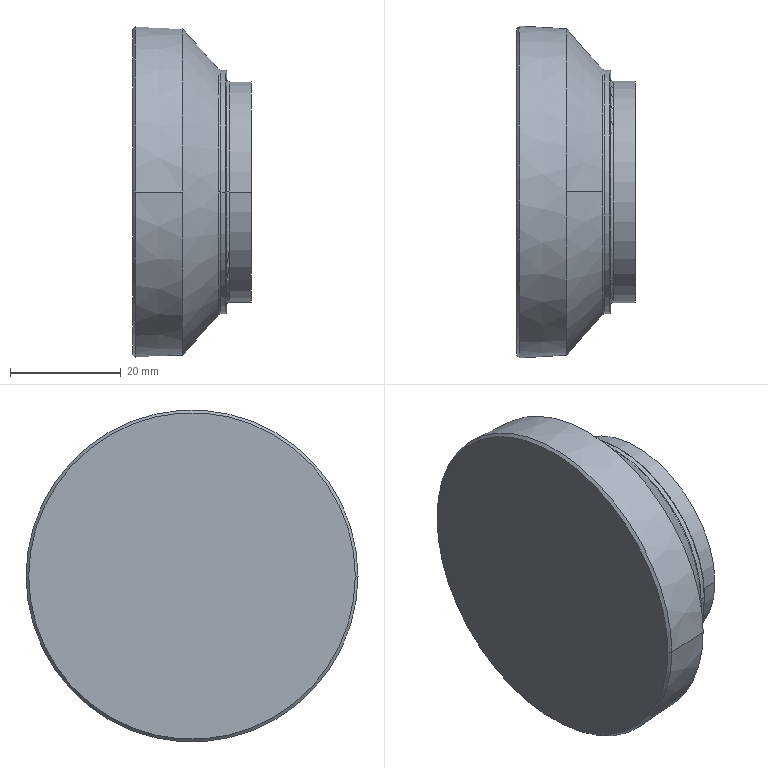Part | SolidWorks | features BaseBody 1 | 1 solid | 23 faces | box 21.5 x 60 x 60 mm | volume 41869 mm3 | torus 6 | cone 6 | cylinder 6 | plane 3 | sphere 2 | commonest cylinder face diameters 22 x2 40 x2 44 x2
STEP:
#1=CARTESIAN_POINT('',(-11.027,-22.,0.));
#2=VERTEX_POINT('',#1);
#3=CARTESIAN_POINT('',(-11.027,22.,0.));
#4=VERTEX_POINT('',#3);
#5=CARTESIAN_POINT('',(-11.027,0.,0.));
#6=DIRECTION('',(1.,0.,0.));
#7=DIRECTION('',(0.,0.,-1.));
#8=AXIS2_PLACEMENT_3D('',#5,#6,#7);
#9=CIRCLE('',#8,22.);
#10=EDGE_CURVE('',#2,#4,#9,.T.);
#11=ORIENTED_EDGE('',*,*,#10,.F.);
#12=CARTESIAN_POINT('',(-11.399,-22.166,0.));
#13=VERTEX_POINT('',#12);
#14=CARTESIAN_POINT('',(-11.027,-22.5,0.));
#15=DIRECTION('',(0.,0.,1.));
#16=DIRECTION('',(0.,-1.,0.));
#17=AXIS2_PLACEMENT_3D('',#14,#15,#16);
#18=CIRCLE('',#17,0.5);
#19=EDGE_CURVE('',#2,#13,#18,.T.);
#20=ORIENTED_EDGE('',*,*,#19,.T.);
#21=CARTESIAN_POINT('',(-11.399,0.,-22.166));
#22=VERTEX_POINT('',#21);
#23=CARTESIAN_POINT('',(-11.399,0.,0.));
#24=DIRECTION('',(-1.,0.,0.));
#25=DIRECTION('',(0.,-1.,0.));
#26=AXIS2_PLACEMENT_3D('',#23,#24,#25);
#27=CIRCLE('',#26,22.166);
#28=EDGE_CURVE('',#22,#13,#27,.T.);
#29=ORIENTED_EDGE('',*,*,#28,.F.);
#30=CARTESIAN_POINT('',(-11.399,22.166,0.));
#31=VERTEX_POINT('',#30);
#32=CARTESIAN_POINT('',(-11.399,0.,0.));
#33=DIRECTION('',(-1.,0.,0.));
#34=DIRECTION('',(0.,-1.,0.));
#35=AXIS2_PLACEMENT_3D('',#32,#33,#34);
#36=CIRCLE('',#35,22.166);
#37=EDGE_CURVE('',#31,#22,#36,.T.);
#38=ORIENTED_EDGE('',*,*,#37,.F.);
#39=CARTESIAN_POINT('',(-11.027,22.5,0.));
#40=DIRECTION('',(0.,0.,-1.));
#41=DIRECTION('',(-1.,0.,0.));
#42=AXIS2_PLACEMENT_3D('',#39,#40,#41);
#43=CIRCLE('',#42,0.5);
#44=EDGE_CURVE('',#4,#31,#43,.T.);
#45=ORIENTED_EDGE('',*,*,#44,.F.);
#46=EDGE_LOOP('',(#11,#20,#29,#38,#45));
#47=FACE_OUTER_BOUND('',#46,.T.);
#48=CARTESIAN_POINT('',(-11.027,0.,0.));
#49=DIRECTION('',(1.,0.,0.));
#50=DIRECTION('',(0.,1.,0.));
#51=AXIS2_PLACEMENT_3D('',#48,#49,#50);
#52=TOROIDAL_SURFACE('',#51,22.5,0.5);
#53=ADVANCED_FACE('',(#47),#52,.F.);
#54=CARTESIAN_POINT('',(-10.2,-22.,0.));
#55=VERTEX_POINT('',#54);
#56=CARTESIAN_POINT('',(-10.2,22.,0.));
#57=VERTEX_POINT('',#56);
#58=CARTESIAN_POINT('',(-10.2,0.,0.));
#59=DIRECTION('',(-1.,0.,0.));
#60=DIRECTION('',(0.,-1.,0.));
#61=AXIS2_PLACEMENT_3D('',#58,#59,#60);
#62=CIRCLE('',#61,22.);
#63=EDGE_CURVE('',#55,#57,#62,.T.);
#64=ORIENTED_EDGE('',*,*,#63,.F.);
#65=CARTESIAN_POINT('',(-10.,-21.8,0.));
#66=VERTEX_POINT('',#65);
#67=CARTESIAN_POINT('',(-10.2,-21.8,0.));
#68=DIRECTION('',(0.,0.,1.));
#69=DIRECTION('',(0.,-1.,0.));
#70=AXIS2_PLACEMENT_3D('',#67,#68,#69);
#71=CIRCLE('',#70,0.2);
#72=EDGE_CURVE('',#55,#66,#71,.T.);
#73=ORIENTED_EDGE('',*,*,#72,.T.);
#74=CARTESIAN_POINT('',(-10.,21.8,0.));
#75=VERTEX_POINT('',#74);
#76=CARTESIAN_POINT('',(-10.,0.,0.));
#77=DIRECTION('',(-1.,0.,0.));
#78=DIRECTION('',(0.,-1.,0.));
#79=AXIS2_PLACEMENT_3D('',#76,#77,#78);
#80=CIRCLE('',#79,21.8);
#81=EDGE_CURVE('',#66,#75,#80,.T.);
#82=ORIENTED_EDGE('',*,*,#81,.T.);
#83=CARTESIAN_POINT('',(-10.2,21.8,0.));
#84=DIRECTION('',(0.,0.,-1.));
#85=DIRECTION('',(-1.,0.,0.));
#86=AXIS2_PLACEMENT_3D('',#83,#84,#85);
#87=CIRCLE('',#86,0.2);
#88=EDGE_CURVE('',#57,#75,#87,.T.);
#89=ORIENTED_EDGE('',*,*,#88,.F.);
#90=EDGE_LOOP('',(#64,#73,#82,#89));
#91=FACE_OUTER_BOUND('',#90,.T.);
#92=CARTESIAN_POINT('',(-10.2,0.,0.));
#93=DIRECTION('',(1.,0.,0.));
#94=DIRECTION('',(0.,1.,0.));
#95=AXIS2_PLACEMENT_3D('',#92,#93,#94);
#96=TOROIDAL_SURFACE('',#95,21.8,0.2);
#97=ADVANCED_FACE('',(#91),#96,.T.);
#98=CARTESIAN_POINT('',(-9.5,-20.,0.));
#99=VERTEX_POINT('',#98);
#100=CARTESIAN_POINT('',(-9.5,20.,0.));
#101=VERTEX_POINT('',#100);
#102=CARTESIAN_POINT('',(-9.5,0.,0.));
#103=DIRECTION('',(1.,0.,0.));
#104=DIRECTION('',(0.,0.,-1.));
#105=AXIS2_PLACEMENT_3D('',#102,#103,#104);
#106=CIRCLE('',#105,20.);
#107=EDGE_CURVE('',#99,#101,#106,.T.);
#108=ORIENTED_EDGE('',*,*,#107,.F.);
#109=CARTESIAN_POINT('',(-10.,-20.5,0.));
#110=VERTEX_POINT('',#109);
#111=CARTESIAN_POINT('',(-9.5,-20.5,0.));
#112=DIRECTION('',(0.,0.,1.));
#113=DIRECTION('',(0.,-1.,0.));
#114=AXIS2_PLACEMENT_3D('',#111,#112,#113);
#115=CIRCLE('',#114,0.5);
#116=EDGE_CURVE('',#99,#110,#115,.T.);
#117=ORIENTED_EDGE('',*,*,#116,.T.);
#118=CARTESIAN_POINT('',(-10.,0.,-20.5));
#119=VERTEX_POINT('',#118);
#120=CARTESIAN_POINT('',(-10.,0.,-20.5));
#121=CARTESIAN_POINT('',(-10.,-0.627,-20.5));
#122=CARTESIAN_POINT('',(-10.,-1.564,-20.457));
#123=CARTESIAN_POINT('',(-10.,-2.649,-20.332));
#124=CARTESIAN_POINT('',(-10.,-3.19,-20.251));
#125=CARTESIAN_POINT('',(-10.,-3.46,-20.206));
#126=CARTESIAN_POINT('',(-10.,-3.595,-20.182));
#127=CARTESIAN_POINT('',(-10.,-3.653,-20.172));
#128=CARTESIAN_POINT('',(-10.,-3.692,-20.165));
#129=CARTESIAN_POINT('',(-10.,-3.71,-20.162));
#130=CARTESIAN_POINT('',(-10.,-4.384,-20.037));
#131=CARTESIAN_POINT('',(-10.,-5.351,-19.809));
#132=CARTESIAN_POINT('',(-10.,-6.456,-19.462));
#133=CARTESIAN_POINT('',(-10.,-7.003,-19.268));
#134=CARTESIAN_POINT('',(-10.,-7.275,-19.166));
#135=CARTESIAN_POINT('',(-10.,-7.391,-19.121));
#136=CARTESIAN_POINT('',(-10.,-7.469,-19.091));
#137=CARTESIAN_POINT('',(-10.,-7.506,-19.077));
#138=CARTESIAN_POINT('',(-10.,-8.19,-18.806));
#139=CARTESIAN_POINT('',(-10.,-9.132,-18.377));
#140=CARTESIAN_POINT('',(-10.,-10.189,-17.795));
#141=CARTESIAN_POINT('',(-10.,-10.707,-17.483));
#142=CARTESIAN_POINT('',(-10.,-10.927,-17.346));
#143=CARTESIAN_POINT('',(-10.,-11.073,-17.253));
#144=CARTESIAN_POINT('',(-10.,-11.144,-17.207));
#145=CARTESIAN_POINT('',(-10.,-12.402,-16.384));
#146=CARTESIAN_POINT('',(-10.,-13.495,-15.496));
#147=CARTESIAN_POINT('',(-10.,-14.996,-13.995));
#148=CARTESIAN_POINT('',(-10.,-15.704,-13.211));
#149=CARTESIAN_POINT('',(-10.,-16.456,-12.234));
#150=CARTESIAN_POINT('',(-10.,-16.813,-11.731));
#151=CARTESIAN_POINT('',(-10.,-16.963,-11.512));
#152=CARTESIAN_POINT('',(-10.,-17.061,-11.366));
#153=CARTESIAN_POINT('',(-10.,-17.111,-11.29));
#154=CARTESIAN_POINT('',(-10.,-17.537,-10.638));
#155=CARTESIAN_POINT('',(-10.,-18.059,-9.744));
#156=CARTESIAN_POINT('',(-10.,-18.587,-8.659));
#157=CARTESIAN_POINT('',(-10.,-18.831,-8.106));
#158=CARTESIAN_POINT('',(-10.,-18.947,-7.827));
#159=CARTESIAN_POINT('',(-10.,-18.996,-7.707));
#160=CARTESIAN_POINT('',(-10.,-19.029,-7.626));
#161=CARTESIAN_POINT('',(-10.,-19.045,-7.585));
#162=CARTESIAN_POINT('',(-10.,-19.305,-6.928));
#163=CARTESIAN_POINT('',(-10.,-19.626,-5.987));
#164=CARTESIAN_POINT('',(-10.,-19.919,-4.867));
#165=CARTESIAN_POINT('',(-10.,-20.045,-4.3));
#166=CARTESIAN_POINT('',(-10.,-20.103,-4.016));
#167=CARTESIAN_POINT('',(-10.,-20.131,-3.873));
#168=CARTESIAN_POINT('',(-10.,-20.142,-3.812));
#169=CARTESIAN_POINT('',(-10.,-20.15,-3.771));
#170=CARTESIAN_POINT('',(-10.,-20.154,-3.749));
#171=CARTESIAN_POINT('',(-10.,-20.386,-2.498));
#172=CARTESIAN_POINT('',(-10.,-20.5,-1.254));
#173=CARTESIAN_POINT('',(-10.,-20.5,0.));
#174=B_SPLINE_CURVE_WITH_KNOTS('',3,(#120,#121,#122,#123,#124,#125,#126,#127,#128,#129,#130,#131,#132,#133,#134,#135,#136,#137,#138,#139,#140,#141,#142,#143,#144,#145,#146,#147,#148,#149,#150,#151,#152,#153,#154,#155,#156,#157,#158,#159,#160,#161,#162,#163,#164,#165,#166,#167,#168,#169,#170,#171,#172,#173),.UNSPECIFIED.,.F.,.F.,(4,1,1,1,1,1,2,2,1,1,1,1,2,2,1,1,1,2,2,2,1,1,1,2,2,1,1,1,1,2,2,1,1,1,1,1,2,2,4),(0.,0.0625,0.09375,0.1094,0.1172,0.1211,0.123,0.125,0.1875,0.2187,0.2344,0.2422,0.2461,0.25,0.3125,0.3437,0.3594,0.3672,0.375,0.5,0.5625,0.5938,0.6094,0.6172,0.625,0.6875,0.7188,0.7344,0.7422,0.7461,0.75,0.8125,0.8438,0.8594,0.8672,0.8711,0.873,0.875,1.),.UNSPECIFIED.);
#175=EDGE_CURVE('',#119,#110,#174,.T.);
#176=ORIENTED_EDGE('',*,*,#175,.F.);
#177=CARTESIAN_POINT('',(-10.,20.5,0.));
#178=VERTEX_POINT('',#177);
#179=CARTESIAN_POINT('',(-10.,20.5,0.));
#180=CARTESIAN_POINT('',(-10.,20.5,-0.6268));
#181=CARTESIAN_POINT('',(-10.,20.457,-1.563));
#182=CARTESIAN_POINT('',(-10.,20.332,-2.649));
#183=CARTESIAN_POINT('',(-10.,20.251,-3.19));
#184=CARTESIAN_POINT('',(-10.,20.206,-3.46));
#185=CARTESIAN_POINT('',(-10.,20.182,-3.595));
#186=CARTESIAN_POINT('',(-10.,20.172,-3.653));
#187=CARTESIAN_POINT('',(-10.,20.165,-3.692));
#188=CARTESIAN_POINT('',(-10.,20.162,-3.71));
#189=CARTESIAN_POINT('',(-10.,20.037,-4.384));
#190=CARTESIAN_POINT('',(-10.,19.809,-5.351));
#191=CARTESIAN_POINT('',(-10.,19.462,-6.456));
#192=CARTESIAN_POINT('',(-10.,19.268,-7.003));
#193=CARTESIAN_POINT('',(-10.,19.166,-7.275));
#194=CARTESIAN_POINT('',(-10.,19.121,-7.391));
#195=CARTESIAN_POINT('',(-10.,19.091,-7.469));
#196=CARTESIAN_POINT('',(-10.,19.077,-7.506));
#197=CARTESIAN_POINT('',(-10.,18.806,-8.19));
#198=CARTESIAN_POINT('',(-10.,18.377,-9.132));
#199=CARTESIAN_POINT('',(-10.,17.795,-10.189));
#200=CARTESIAN_POINT('',(-10.,17.483,-10.707));
#201=CARTESIAN_POINT('',(-10.,17.346,-10.927));
#202=CARTESIAN_POINT('',(-10.,17.253,-11.073));
#203=CARTESIAN_POINT('',(-10.,17.207,-11.144));
#204=CARTESIAN_POINT('',(-10.,16.384,-12.402));
#205=CARTESIAN_POINT('',(-10.,15.496,-13.495));
#206=CARTESIAN_POINT('',(-10.,13.995,-14.996));
#207=CARTESIAN_POINT('',(-10.,13.211,-15.704));
#208=CARTESIAN_POINT('',(-10.,12.234,-16.456));
#209=CARTESIAN_POINT('',(-10.,11.731,-16.813));
#210=CARTESIAN_POINT('',(-10.,11.512,-16.963));
#211=CARTESIAN_POINT('',(-10.,11.366,-17.061));
#212=CARTESIAN_POINT('',(-10.,11.29,-17.111));
#213=CARTESIAN_POINT('',(-10.,10.638,-17.537));
#214=CARTESIAN_POINT('',(-10.,9.744,-18.059));
#215=CARTESIAN_POINT('',(-10.,8.659,-18.587));
#216=CARTESIAN_POINT('',(-10.,8.106,-18.831));
#217=CARTESIAN_POINT('',(-10.,7.827,-18.947));
#218=CARTESIAN_POINT('',(-10.,7.707,-18.996));
#219=CARTESIAN_POINT('',(-10.,7.626,-19.029));
#220=CARTESIAN_POINT('',(-10.,7.585,-19.045));
#221=CARTESIAN_POINT('',(-10.,6.928,-19.305));
#222=CARTESIAN_POINT('',(-10.,5.987,-19.626));
#223=CARTESIAN_POINT('',(-10.,4.867,-19.919));
#224=CARTESIAN_POINT('',(-10.,4.3,-20.045));
#225=CARTESIAN_POINT('',(-10.,4.016,-20.103));
#226=CARTESIAN_POINT('',(-10.,3.873,-20.131));
#227=CARTESIAN_POINT('',(-10.,3.812,-20.142));
#228=CARTESIAN_POINT('',(-10.,3.771,-20.15));
#229=CARTESIAN_POINT('',(-10.,3.749,-20.154));
#230=CARTESIAN_POINT('',(-10.,2.498,-20.386));
#231=CARTESIAN_POINT('',(-10.,1.254,-20.5));
#232=CARTESIAN_POINT('',(-10.,0.,-20.5));
#233=B_SPLINE_CURVE_WITH_KNOTS('',3,(#179,#180,#181,#182,#183,#184,#185,#186,#187,#188,#189,#190,#191,#192,#193,#194,#195,#196,#197,#198,#199,#200,#201,#202,#203,#204,#205,#206,#207,#208,#209,#210,#211,#212,#213,#214,#215,#216,#217,#218,#219,#220,#221,#222,#223,#224,#225,#226,#227,#228,#229,#230,#231,#232),.UNSPECIFIED.,.F.,.F.,(4,1,1,1,1,1,2,2,1,1,1,1,2,2,1,1,1,2,2,2,1,1,1,2,2,1,1,1,1,2,2,1,1,1,1,1,2,2,4),(0.5,0.5312,0.5469,0.5547,0.5586,0.5605,0.5615,0.5625,0.5937,0.6094,0.6172,0.6211,0.623,0.625,0.6562,0.6719,0.6797,0.6836,0.6875,0.75,0.7812,0.7969,0.8047,0.8086,0.8125,0.8437,0.8594,0.8672,0.8711,0.873,0.875,0.9062,0.9219,0.9297,0.9336,0.9355,0.9365,0.9375,1.),.UNSPECIFIED.);
#234=EDGE_CURVE('',#178,#119,#233,.T.);
#235=ORIENTED_EDGE('',*,*,#234,.F.);
#236=CARTESIAN_POINT('',(-9.5,20.5,0.));
#237=DIRECTION('',(0.,0.,-1.));
#238=DIRECTION('',(-1.,0.,0.));
#239=AXIS2_PLACEMENT_3D('',#236,#237,#238);
#240=CIRCLE('',#239,0.5);
#241=EDGE_CURVE('',#101,#178,#240,.T.);
#242=ORIENTED_EDGE('',*,*,#241,.F.);
#243=EDGE_LOOP('',(#108,#117,#176,#235,#242));
#244=FACE_OUTER_BOUND('',#243,.T.);
#245=CARTESIAN_POINT('',(-9.5,0.,0.));
#246=DIRECTION('',(1.,0.,0.));
#247=DIRECTION('',(0.,1.,0.));
#248=AXIS2_PLACEMENT_3D('',#245,#246,#247);
#249=TOROIDAL_SURFACE('',#248,20.5,0.5);
#250=ADVANCED_FACE('',(#244),#249,.F.);
#251=CARTESIAN_POINT('',(-22.,0.,0.));
#252=VERTEX_POINT('',#251);
#253=CARTESIAN_POINT('',(-11.,11.,0.));
#254=VERTEX_POINT('',#253);
#255=CARTESIAN_POINT('',(-11.,0.,0.));
#256=DIRECTION('',(0.,0.,-1.));
#257=DIRECTION('',(-1.,0.,0.));
#258=AXIS2_PLACEMENT_3D('',#255,#256,#257);
#259=CIRCLE('',#258,11.);
#260=EDGE_CURVE('',#252,#254,#259,.T.);
#261=ORIENTED_EDGE('',*,*,#260,.F.);
#262=CARTESIAN_POINT('',(-11.,-11.,0.));
#263=VERTEX_POINT('',#262);
#264=CARTESIAN_POINT('',(-11.,0.,0.));
#265=DIRECTION('',(0.,0.,1.));
#266=DIRECTION('',(1.,0.,0.));
#267=AXIS2_PLACEMENT_3D('',#264,#265,#266);
#268=CIRCLE('',#267,11.);
#269=EDGE_CURVE('',#252,#263,#268,.T.);
#270=ORIENTED_EDGE('',*,*,#269,.T.);
#271=CARTESIAN_POINT('',(-11.,0.,0.));
#272=DIRECTION('',(1.,0.,0.));
#273=DIRECTION('',(0.,-1.,0.));
#274=AXIS2_PLACEMENT_3D('',#271,#272,#273);
#275=CIRCLE('',#274,11.);
#276=EDGE_CURVE('',#263,#254,#275,.T.);
#277=ORIENTED_EDGE('',*,*,#276,.T.);
#278=EDGE_LOOP('',(#261,#270,#277));
#279=FACE_OUTER_BOUND('',#278,.T.);
#280=CARTESIAN_POINT('',(-11.,0.,0.));
#281=DIRECTION('',(0.,0.,1.));
#282=DIRECTION('',(0.,1.,0.));
#283=AXIS2_PLACEMENT_3D('',#280,#281,#282);
#284=SPHERICAL_SURFACE('',#283,11.);
#285=ADVANCED_FACE('',(#279),#284,.F.);
#286=CARTESIAN_POINT('',(-27.,-29.5,0.));
#287=VERTEX_POINT('',#286);
#288=CARTESIAN_POINT('',(-27.,29.5,0.));
#289=VERTEX_POINT('',#288);
#290=CARTESIAN_POINT('',(-27.,0.,0.));
#291=DIRECTION('',(-1.,0.,0.));
#292=DIRECTION('',(0.,0.,-1.));
#293=AXIS2_PLACEMENT_3D('',#290,#291,#292);
#294=CIRCLE('',#293,29.5);
#295=EDGE_CURVE('',#287,#289,#294,.T.);
#296=ORIENTED_EDGE('',*,*,#295,.F.);
#297=CARTESIAN_POINT('',(-26.5,-30.,0.));
#298=VERTEX_POINT('',#297);
#299=CARTESIAN_POINT('',(-26.5,-30.,0.));
#300=DIRECTION('',(0.7071,-0.7071,0.));
#301=VECTOR('',#300,1000.);
#302=LINE('',#299,#301);
#303=EDGE_CURVE('',#287,#298,#302,.T.);
#304=ORIENTED_EDGE('',*,*,#303,.T.);
#305=CARTESIAN_POINT('',(-26.5,30.,0.));
#306=VERTEX_POINT('',#305);
#307=CARTESIAN_POINT('',(-26.5,0.,0.));
#308=DIRECTION('',(-1.,0.,0.));
#309=DIRECTION('',(0.,-1.,0.));
#310=AXIS2_PLACEMENT_3D('',#307,#308,#309);
#311=CIRCLE('',#310,30.);
#312=EDGE_CURVE('',#298,#306,#311,.T.);
#313=ORIENTED_EDGE('',*,*,#312,.T.);
#314=CARTESIAN_POINT('',(-26.5,30.,0.));
#315=DIRECTION('',(0.7071,0.7071,0.));
#316=VECTOR('',#315,1000.);
#317=LINE('',#314,#316);
#318=EDGE_CURVE('',#289,#306,#317,.T.);
#319=ORIENTED_EDGE('',*,*,#318,.F.);
#320=EDGE_LOOP('',(#296,#304,#313,#319));
#321=FACE_OUTER_BOUND('',#320,.T.);
#322=CARTESIAN_POINT('',(-26.5,0.,0.));
#323=DIRECTION('',(1.,0.,0.));
#324=DIRECTION('',(0.,1.,0.));
#325=AXIS2_PLACEMENT_3D('',#322,#323,#324);
#326=CONICAL_SURFACE('',#325,30.,0.7854);
#327=ADVANCED_FACE('',(#321),#326,.T.);
#328=CARTESIAN_POINT('',(-18.,0.,29.5));
#329=VERTEX_POINT('',#328);
#330=CARTESIAN_POINT('',(-18.,29.5,0.));
#331=VERTEX_POINT('',#330);
#332=CARTESIAN_POINT('',(-18.,0.,0.));
#333=DIRECTION('',(-1.,0.,0.));
#334=DIRECTION('',(0.,-1.,0.));
#335=AXIS2_PLACEMENT_3D('',#332,#333,#334);
#336=CIRCLE('',#335,29.5);
#337=EDGE_CURVE('',#329,#331,#336,.T.);
#338=ORIENTED_EDGE('',*,*,#337,.T.);
#339=CARTESIAN_POINT('',(-26.5,30.,0.));
#340=DIRECTION('',(-0.9983,0.05872,0.));
#341=VECTOR('',#340,1000.);
#342=LINE('',#339,#341);
#343=EDGE_CURVE('',#331,#306,#342,.T.);
#344=ORIENTED_EDGE('',*,*,#343,.T.);
#345=ORIENTED_EDGE('',*,*,#312,.F.);
#346=CARTESIAN_POINT('',(-18.,-29.5,0.));
#347=VERTEX_POINT('',#346);
#348=CARTESIAN_POINT('',(-26.5,-30.,0.));
#349=DIRECTION('',(-0.9983,-0.05872,0.));
#350=VECTOR('',#349,1000.);
#351=LINE('',#348,#350);
#352=EDGE_CURVE('',#347,#298,#351,.T.);
#353=ORIENTED_EDGE('',*,*,#352,.F.);
#354=CARTESIAN_POINT('',(-18.,0.,0.));
#355=DIRECTION('',(-1.,0.,0.));
#356=DIRECTION('',(0.,-1.,0.));
#357=AXIS2_PLACEMENT_3D('',#354,#355,#356);
#358=CIRCLE('',#357,29.5);
#359=EDGE_CURVE('',#347,#329,#358,.T.);
#360=ORIENTED_EDGE('',*,*,#359,.T.);
#361=EDGE_LOOP('',(#338,#344,#345,#353,#360));
#362=FACE_OUTER_BOUND('',#361,.T.);
#363=CARTESIAN_POINT('',(-26.5,0.,0.));
#364=DIRECTION('',(-1.,0.,0.));
#365=DIRECTION('',(0.,-1.,0.));
#366=AXIS2_PLACEMENT_3D('',#363,#364,#365);
#367=CONICAL_SURFACE('',#366,30.,0.05876);
#368=ADVANCED_FACE('',(#362),#367,.T.);
#369=CARTESIAN_POINT('',(-11.399,0.,22.166));
#370=VERTEX_POINT('',#369);
#371=CARTESIAN_POINT('',(-11.399,0.,0.));
#372=DIRECTION('',(-1.,0.,0.));
#373=DIRECTION('',(0.,-1.,0.));
#374=AXIS2_PLACEMENT_3D('',#371,#372,#373);
#375=CIRCLE('',#374,22.166);
#376=EDGE_CURVE('',#370,#31,#375,.T.);
#377=ORIENTED_EDGE('',*,*,#376,.T.);
#378=ORIENTED_EDGE('',*,*,#37,.T.);
#379=CARTESIAN_POINT('',(-18.,0.,-29.5));
#380=VERTEX_POINT('',#379);
#381=CARTESIAN_POINT('',(-18.,0.,-29.5));
#382=DIRECTION('',(-0.669,0.,-0.7433));
#383=VECTOR('',#382,1000.);
#384=LINE('',#381,#383);
#385=EDGE_CURVE('',#22,#380,#384,.T.);
#386=ORIENTED_EDGE('',*,*,#385,.T.);
#387=CARTESIAN_POINT('',(-18.,0.,0.));
#388=DIRECTION('',(-1.,0.,0.));
#389=DIRECTION('',(0.,-1.,0.));
#390=AXIS2_PLACEMENT_3D('',#387,#388,#389);
#391=CIRCLE('',#390,29.5);
#392=EDGE_CURVE('',#331,#380,#391,.T.);
#393=ORIENTED_EDGE('',*,*,#392,.F.);
#394=ORIENTED_EDGE('',*,*,#337,.F.);
#395=CARTESIAN_POINT('',(-18.,0.,29.5));
#396=DIRECTION('',(-0.669,0.,0.7433));
#397=VECTOR('',#396,1000.);
#398=LINE('',#395,#397);
#399=EDGE_CURVE('',#370,#329,#398,.T.);
#400=ORIENTED_EDGE('',*,*,#399,.F.);
#401=EDGE_LOOP('',(#377,#378,#386,#393,#394,#400));
#402=FACE_OUTER_BOUND('',#401,.T.);
#403=CARTESIAN_POINT('',(-18.,0.,0.));
#404=DIRECTION('',(-1.,0.,0.));
#405=DIRECTION('',(0.,0.,1.));
#406=AXIS2_PLACEMENT_3D('',#403,#404,#405);
#407=CONICAL_SURFACE('',#406,29.5,0.838);
#408=ADVANCED_FACE('',(#402),#407,.T.);
#409=ORIENTED_EDGE('',*,*,#63,.T.);
#410=CARTESIAN_POINT('',(-10.614,22.,0.));
#411=DIRECTION('',(-1.,0.,0.));
#412=VECTOR('',#411,1000.);
#413=LINE('',#410,#412);
#414=EDGE_CURVE('',#57,#4,#413,.T.);
#415=ORIENTED_EDGE('',*,*,#414,.T.);
#416=CARTESIAN_POINT('',(-11.027,0.,0.));
#417=DIRECTION('',(1.,0.,0.));
#418=DIRECTION('',(0.,0.,-1.));
#419=AXIS2_PLACEMENT_3D('',#416,#417,#418);
#420=CIRCLE('',#419,22.);
#421=EDGE_CURVE('',#4,#2,#420,.T.);
#422=ORIENTED_EDGE('',*,*,#421,.T.);
#423=CARTESIAN_POINT('',(-10.614,-22.,0.));
#424=DIRECTION('',(-1.,0.,0.));
#425=VECTOR('',#424,1000.);
#426=LINE('',#423,#425);
#427=EDGE_CURVE('',#55,#2,#426,.T.);
#428=ORIENTED_EDGE('',*,*,#427,.F.);
#429=EDGE_LOOP('',(#409,#415,#422,#428));
#430=FACE_OUTER_BOUND('',#429,.T.);
#431=CARTESIAN_POINT('',(-10.614,0.,0.));
#432=DIRECTION('',(-1.,0.,0.));
#433=DIRECTION('',(0.,-1.,0.));
#434=AXIS2_PLACEMENT_3D('',#431,#432,#433);
#435=CYLINDRICAL_SURFACE('',#434,22.);
#436=ADVANCED_FACE('',(#430),#435,.T.);
#437=CARTESIAN_POINT('',(-5.5,-20.,0.));
#438=VERTEX_POINT('',#437);
#439=CARTESIAN_POINT('',(-5.5,20.,0.));
#440=VERTEX_POINT('',#439);
#441=CARTESIAN_POINT('',(-5.5,0.,0.));
#442=DIRECTION('',(-1.,0.,0.));
#443=DIRECTION('',(0.,-1.,0.));
#444=AXIS2_PLACEMENT_3D('',#441,#442,#443);
#445=CIRCLE('',#444,20.);
#446=EDGE_CURVE('',#438,#440,#445,.T.);
#447=ORIENTED_EDGE('',*,*,#446,.T.);
#448=CARTESIAN_POINT('',(-7.5,20.,0.));
#449=DIRECTION('',(-1.,0.,0.));
#450=VECTOR('',#449,1000.);
#451=LINE('',#448,#450);
#452=EDGE_CURVE('',#440,#101,#451,.T.);
#453=ORIENTED_EDGE('',*,*,#452,.T.);
#454=CARTESIAN_POINT('',(-9.5,0.,0.));
#455=DIRECTION('',(1.,0.,0.));
#456=DIRECTION('',(0.,0.,-1.));
#457=AXIS2_PLACEMENT_3D('',#454,#455,#456);
#458=CIRCLE('',#457,20.);
#459=EDGE_CURVE('',#101,#99,#458,.T.);
#460=ORIENTED_EDGE('',*,*,#459,.T.);
#461=CARTESIAN_POINT('',(-7.5,-20.,0.));
#462=DIRECTION('',(-1.,0.,0.));
#463=VECTOR('',#462,1000.);
#464=LINE('',#461,#463);
#465=EDGE_CURVE('',#438,#99,#464,.T.);
#466=ORIENTED_EDGE('',*,*,#465,.F.);
#467=EDGE_LOOP('',(#447,#453,#460,#466));
#468=FACE_OUTER_BOUND('',#467,.T.);
#469=CARTESIAN_POINT('',(-7.5,0.,0.));
#470=DIRECTION('',(-1.,0.,0.));
#471=DIRECTION('',(0.,-1.,0.));
#472=AXIS2_PLACEMENT_3D('',#469,#470,#471);
#473=CYLINDRICAL_SURFACE('',#472,20.);
#474=ADVANCED_FACE('',(#468),#473,.T.);
#475=CARTESIAN_POINT('',(-5.5,11.,0.));
#476=VERTEX_POINT('',#475);
#477=CARTESIAN_POINT('',(-5.5,-11.,0.));
#478=VERTEX_POINT('',#477);
#479=CARTESIAN_POINT('',(-5.5,0.,0.));
#480=DIRECTION('',(-1.,0.,0.));
#481=DIRECTION('',(0.,-1.,0.));
#482=AXIS2_PLACEMENT_3D('',#479,#480,#481);
#483=CIRCLE('',#482,11.);
#484=EDGE_CURVE('',#476,#478,#483,.T.);
#485=ORIENTED_EDGE('',*,*,#484,.F.);
#486=CARTESIAN_POINT('',(-8.25,11.,0.));
#487=DIRECTION('',(-1.,0.,0.));
#488=VECTOR('',#487,1000.);
#489=LINE('',#486,#488);
#490=EDGE_CURVE('',#476,#254,#489,.T.);
#491=ORIENTED_EDGE('',*,*,#490,.T.);
#492=ORIENTED_EDGE('',*,*,#276,.F.);
#493=CARTESIAN_POINT('',(-8.25,-11.,0.));
#494=DIRECTION('',(-1.,0.,0.));
#495=VECTOR('',#494,1000.);
#496=LINE('',#493,#495);
#497=EDGE_CURVE('',#478,#263,#496,.T.);
#498=ORIENTED_EDGE('',*,*,#497,.F.);
#499=EDGE_LOOP('',(#485,#491,#492,#498));
#500=FACE_OUTER_BOUND('',#499,.T.);
#501=CARTESIAN_POINT('',(-8.25,0.,0.));
#502=DIRECTION('',(-1.,0.,0.));
#503=DIRECTION('',(0.,-1.,0.));
#504=AXIS2_PLACEMENT_3D('',#501,#502,#503);
#505=CYLINDRICAL_SURFACE('',#504,11.);
#506=ADVANCED_FACE('',(#500),#505,.F.);
#507=CARTESIAN_POINT('',(-5.5,0.,0.));
#508=DIRECTION('',(-1.,0.,0.));
#509=DIRECTION('',(0.,-1.,0.));
#510=AXIS2_PLACEMENT_3D('',#507,#508,#509);
#511=CIRCLE('',#510,11.);
#512=EDGE_CURVE('',#478,#476,#511,.T.);
#513=ORIENTED_EDGE('',*,*,#512,.T.);
#514=ORIENTED_EDGE('',*,*,#484,.T.);
#515=EDGE_LOOP('',(#513,#514));
#516=FACE_BOUND('',#515,.T.);
#517=ORIENTED_EDGE('',*,*,#446,.F.);
#518=CARTESIAN_POINT('',(-5.5,0.,0.));
#519=DIRECTION('',(-1.,0.,0.));
#520=DIRECTION('',(0.,-1.,0.));
#521=AXIS2_PLACEMENT_3D('',#518,#519,#520);
#522=CIRCLE('',#521,20.);
#523=EDGE_CURVE('',#440,#438,#522,.T.);
#524=ORIENTED_EDGE('',*,*,#523,.F.);
#525=EDGE_LOOP('',(#517,#524));
#526=FACE_OUTER_BOUND('',#525,.T.);
#527=CARTESIAN_POINT('',(-5.5,-15.5,0.));
#528=DIRECTION('',(1.,0.,0.));
#529=DIRECTION('',(0.,0.,-1.));
#530=AXIS2_PLACEMENT_3D('',#527,#528,#529);
#531=PLANE('',#530);
#532=ADVANCED_FACE('',(#516,#526),#531,.T.);
#533=CARTESIAN_POINT('',(-10.,0.,20.5));
#534=VERTEX_POINT('',#533);
#535=CARTESIAN_POINT('',(-10.,-20.5,0.));
#536=CARTESIAN_POINT('',(-10.,-20.5,0.627));
#537=CARTESIAN_POINT('',(-10.,-20.457,1.564));
#538=CARTESIAN_POINT('',(-10.,-20.332,2.649));
#539=CARTESIAN_POINT('',(-10.,-20.251,3.19));
#540=CARTESIAN_POINT('',(-10.,-20.206,3.46));
#541=CARTESIAN_POINT('',(-10.,-20.182,3.595));
#542=CARTESIAN_POINT('',(-10.,-20.172,3.653));
#543=CARTESIAN_POINT('',(-10.,-20.165,3.692));
#544=CARTESIAN_POINT('',(-10.,-20.162,3.71));
#545=CARTESIAN_POINT('',(-10.,-20.037,4.384));
#546=CARTESIAN_POINT('',(-10.,-19.809,5.351));
#547=CARTESIAN_POINT('',(-10.,-19.462,6.456));
#548=CARTESIAN_POINT('',(-10.,-19.268,7.003));
#549=CARTESIAN_POINT('',(-10.,-19.166,7.275));
#550=CARTESIAN_POINT('',(-10.,-19.121,7.391));
#551=CARTESIAN_POINT('',(-10.,-19.091,7.469));
#552=CARTESIAN_POINT('',(-10.,-19.077,7.506));
#553=CARTESIAN_POINT('',(-10.,-18.806,8.19));
#554=CARTESIAN_POINT('',(-10.,-18.377,9.132));
#555=CARTESIAN_POINT('',(-10.,-17.795,10.189));
#556=CARTESIAN_POINT('',(-10.,-17.483,10.707));
#557=CARTESIAN_POINT('',(-10.,-17.346,10.927));
#558=CARTESIAN_POINT('',(-10.,-17.253,11.073));
#559=CARTESIAN_POINT('',(-10.,-17.207,11.144));
#560=CARTESIAN_POINT('',(-10.,-16.384,12.402));
#561=CARTESIAN_POINT('',(-10.,-15.496,13.495));
#562=CARTESIAN_POINT('',(-10.,-13.995,14.996));
#563=CARTESIAN_POINT('',(-10.,-13.211,15.704));
#564=CARTESIAN_POINT('',(-10.,-12.234,16.456));
#565=CARTESIAN_POINT('',(-10.,-11.731,16.813));
#566=CARTESIAN_POINT('',(-10.,-11.512,16.963));
#567=CARTESIAN_POINT('',(-10.,-11.366,17.061));
#568=CARTESIAN_POINT('',(-10.,-11.29,17.111));
#569=CARTESIAN_POINT('',(-10.,-10.638,17.537));
#570=CARTESIAN_POINT('',(-10.,-9.744,18.059));
#571=CARTESIAN_POINT('',(-10.,-8.659,18.587));
#572=CARTESIAN_POINT('',(-10.,-8.106,18.831));
#573=CARTESIAN_POINT('',(-10.,-7.827,18.947));
#574=CARTESIAN_POINT('',(-10.,-7.707,18.996));
#575=CARTESIAN_POINT('',(-10.,-7.626,19.029));
#576=CARTESIAN_POINT('',(-10.,-7.585,19.045));
#577=CARTESIAN_POINT('',(-10.,-6.928,19.305));
#578=CARTESIAN_POINT('',(-10.,-5.987,19.626));
#579=CARTESIAN_POINT('',(-10.,-4.867,19.919));
#580=CARTESIAN_POINT('',(-10.,-4.3,20.045));
#581=CARTESIAN_POINT('',(-10.,-4.016,20.103));
#582=CARTESIAN_POINT('',(-10.,-3.873,20.131));
#583=CARTESIAN_POINT('',(-10.,-3.812,20.142));
#584=CARTESIAN_POINT('',(-10.,-3.771,20.15));
#585=CARTESIAN_POINT('',(-10.,-3.749,20.154));
#586=CARTESIAN_POINT('',(-10.,-2.498,20.386));
#587=CARTESIAN_POINT('',(-10.,-1.254,20.5));
#588=CARTESIAN_POINT('',(-10.,0.,20.5));
#589=B_SPLINE_CURVE_WITH_KNOTS('',3,(#535,#536,#537,#538,#539,#540,#541,#542,#543,#544,#545,#546,#547,#548,#549,#550,#551,#552,#553,#554,#555,#556,#557,#558,#559,#560,#561,#562,#563,#564,#565,#566,#567,#568,#569,#570,#571,#572,#573,#574,#575,#576,#577,#578,#579,#580,#581,#582,#583,#584,#585,#586,#587,#588),.UNSPECIFIED.,.F.,.F.,(4,1,1,1,1,1,2,2,1,1,1,1,2,2,1,1,1,2,2,2,1,1,1,2,2,1,1,1,1,2,2,1,1,1,1,1,2,2,4),(0.,0.0625,0.09375,0.1094,0.1172,0.1211,0.123,0.125,0.1875,0.2188,0.2344,0.2422,0.2461,0.25,0.3125,0.3438,0.3594,0.3672,0.375,0.5,0.5625,0.5938,0.6094,0.6172,0.625,0.6875,0.7188,0.7344,0.7422,0.7461,0.75,0.8125,0.8438,0.8594,0.8672,0.8711,0.873,0.875,1.),.UNSPECIFIED.);
#590=EDGE_CURVE('',#110,#534,#589,.T.);
#591=ORIENTED_EDGE('',*,*,#590,.T.);
#592=CARTESIAN_POINT('',(-10.,0.,20.5));
#593=CARTESIAN_POINT('',(-10.,0.627,20.5));
#594=CARTESIAN_POINT('',(-10.,1.564,20.457));
#595=CARTESIAN_POINT('',(-10.,2.649,20.332));
#596=CARTESIAN_POINT('',(-10.,3.19,20.251));
#597=CARTESIAN_POINT('',(-10.,3.46,20.206));
#598=CARTESIAN_POINT('',(-10.,3.595,20.182));
#599=CARTESIAN_POINT('',(-10.,3.653,20.172));
#600=CARTESIAN_POINT('',(-10.,3.692,20.165));
#601=CARTESIAN_POINT('',(-10.,3.71,20.162));
#602=CARTESIAN_POINT('',(-10.,4.384,20.037));
#603=CARTESIAN_POINT('',(-10.,5.351,19.809));
#604=CARTESIAN_POINT('',(-10.,6.456,19.462));
#605=CARTESIAN_POINT('',(-10.,7.003,19.268));
#606=CARTESIAN_POINT('',(-10.,7.275,19.166));
#607=CARTESIAN_POINT('',(-10.,7.391,19.121));
#608=CARTESIAN_POINT('',(-10.,7.469,19.091));
#609=CARTESIAN_POINT('',(-10.,7.506,19.077));
#610=CARTESIAN_POINT('',(-10.,8.19,18.806));
#611=CARTESIAN_POINT('',(-10.,9.132,18.377));
#612=CARTESIAN_POINT('',(-10.,10.189,17.795));
#613=CARTESIAN_POINT('',(-10.,10.707,17.483));
#614=CARTESIAN_POINT('',(-10.,10.927,17.346));
#615=CARTESIAN_POINT('',(-10.,11.073,17.253));
#616=CARTESIAN_POINT('',(-10.,11.144,17.207));
#617=CARTESIAN_POINT('',(-10.,12.402,16.384));
#618=CARTESIAN_POINT('',(-10.,13.495,15.496));
#619=CARTESIAN_POINT('',(-10.,14.996,13.995));
#620=CARTESIAN_POINT('',(-10.,15.704,13.211));
#621=CARTESIAN_POINT('',(-10.,16.456,12.234));
#622=CARTESIAN_POINT('',(-10.,16.813,11.731));
#623=CARTESIAN_POINT('',(-10.,16.963,11.512));
#624=CARTESIAN_POINT('',(-10.,17.061,11.366));
#625=CARTESIAN_POINT('',(-10.,17.111,11.29));
#626=CARTESIAN_POINT('',(-10.,17.537,10.638));
#627=CARTESIAN_POINT('',(-10.,18.059,9.744));
#628=CARTESIAN_POINT('',(-10.,18.587,8.659));
#629=CARTESIAN_POINT('',(-10.,18.831,8.106));
#630=CARTESIAN_POINT('',(-10.,18.947,7.827));
#631=CARTESIAN_POINT('',(-10.,18.996,7.707));
#632=CARTESIAN_POINT('',(-10.,19.029,7.626));
#633=CARTESIAN_POINT('',(-10.,19.045,7.585));
#634=CARTESIAN_POINT('',(-10.,19.305,6.928));
#635=CARTESIAN_POINT('',(-10.,19.626,5.987));
#636=CARTESIAN_POINT('',(-10.,19.919,4.867));
#637=CARTESIAN_POINT('',(-10.,20.045,4.3));
#638=CARTESIAN_POINT('',(-10.,20.103,4.016));
#639=CARTESIAN_POINT('',(-10.,20.131,3.873));
#640=CARTESIAN_POINT('',(-10.,20.142,3.812));
#641=CARTESIAN_POINT('',(-10.,20.15,3.771));
#642=CARTESIAN_POINT('',(-10.,20.154,3.75));
#643=CARTESIAN_POINT('',(-10.,20.386,2.498));
#644=CARTESIAN_POINT('',(-10.,20.5,1.254));
#645=CARTESIAN_POINT('',(-10.,20.5,0.));
#646=B_SPLINE_CURVE_WITH_KNOTS('',3,(#592,#593,#594,#595,#596,#597,#598,#599,#600,#601,#602,#603,#604,#605,#606,#607,#608,#609,#610,#611,#612,#613,#614,#615,#616,#617,#618,#619,#620,#621,#622,#623,#624,#625,#626,#627,#628,#629,#630,#631,#632,#633,#634,#635,#636,#637,#638,#639,#640,#641,#642,#643,#644,#645),.UNSPECIFIED.,.F.,.F.,(4,1,1,1,1,1,2,2,1,1,1,1,2,2,1,1,1,2,2,2,1,1,1,2,2,1,1,1,1,2,2,1,1,1,1,1,2,2,4),(0.,0.03125,0.04687,0.05469,0.05859,0.06055,0.06152,0.0625,0.09375,0.1094,0.1172,0.1211,0.123,0.125,0.1562,0.1719,0.1797,0.1836,0.1875,0.25,0.2812,0.2969,0.3047,0.3086,0.3125,0.3437,0.3594,0.3672,0.3711,0.373,0.375,0.4062,0.4219,0.4297,0.4336,0.4355,0.4365,0.4375,0.5),.UNSPECIFIED.);
#647=EDGE_CURVE('',#534,#178,#646,.T.);
#648=ORIENTED_EDGE('',*,*,#647,.T.);
#649=ORIENTED_EDGE('',*,*,#234,.T.);
#650=ORIENTED_EDGE('',*,*,#175,.T.);
#651=EDGE_LOOP('',(#591,#648,#649,#650));
#652=FACE_BOUND('',#651,.T.);
#653=CARTESIAN_POINT('',(-10.,0.,0.));
#654=DIRECTION('',(-1.,0.,0.));
#655=DIRECTION('',(0.,-1.,0.));
#656=AXIS2_PLACEMENT_3D('',#653,#654,#655);
#657=CIRCLE('',#656,21.8);
#658=EDGE_CURVE('',#75,#66,#657,.T.);
#659=ORIENTED_EDGE('',*,*,#658,.F.);
#660=ORIENTED_EDGE('',*,*,#81,.F.);
#661=EDGE_LOOP('',(#659,#660));
#662=FACE_OUTER_BOUND('',#661,.T.);
#663=CARTESIAN_POINT('',(-10.,-21.15,0.));
#664=DIRECTION('',(1.,0.,0.));
#665=DIRECTION('',(0.,1.,0.));
#666=AXIS2_PLACEMENT_3D('',#663,#664,#665);
#667=PLANE('',#666);
#668=ADVANCED_FACE('',(#652,#662),#667,.T.);
#669=CARTESIAN_POINT('',(-27.,0.,0.));
#670=DIRECTION('',(-1.,0.,0.));
#671=DIRECTION('',(0.,0.,-1.));
#672=AXIS2_PLACEMENT_3D('',#669,#670,#671);
#673=CIRCLE('',#672,29.5);
#674=EDGE_CURVE('',#289,#287,#673,.T.);
#675=ORIENTED_EDGE('',*,*,#674,.T.);
#676=ORIENTED_EDGE('',*,*,#295,.T.);
#677=EDGE_LOOP('',(#675,#676));
#678=FACE_OUTER_BOUND('',#677,.T.);
#679=CARTESIAN_POINT('',(-27.,-14.75,0.));
#680=DIRECTION('',(-1.,0.,0.));
#681=DIRECTION('',(0.,1.,0.));
#682=AXIS2_PLACEMENT_3D('',#679,#680,#681);
#683=PLANE('',#682);
#684=ADVANCED_FACE('',(#678),#683,.T.);
#685=ORIENTED_EDGE('',*,*,#490,.F.);
#686=ORIENTED_EDGE('',*,*,#512,.F.);
#687=ORIENTED_EDGE('',*,*,#497,.T.);
#688=CARTESIAN_POINT('',(-11.,0.,0.));
#689=DIRECTION('',(1.,0.,0.));
#690=DIRECTION('',(0.,-1.,0.));
#691=AXIS2_PLACEMENT_3D('',#688,#689,#690);
#692=CIRCLE('',#691,11.);
#693=EDGE_CURVE('',#254,#263,#692,.T.);
#694=ORIENTED_EDGE('',*,*,#693,.F.);
#695=EDGE_LOOP('',(#685,#686,#687,#694));
#696=FACE_OUTER_BOUND('',#695,.T.);
#697=CARTESIAN_POINT('',(-8.25,0.,0.));
#698=DIRECTION('',(-1.,0.,0.));
#699=DIRECTION('',(0.,-1.,0.));
#700=AXIS2_PLACEMENT_3D('',#697,#698,#699);
#701=CYLINDRICAL_SURFACE('',#700,11.);
#702=ADVANCED_FACE('',(#696),#701,.F.);
#703=ORIENTED_EDGE('',*,*,#452,.F.);
#704=ORIENTED_EDGE('',*,*,#523,.T.);
#705=ORIENTED_EDGE('',*,*,#465,.T.);
#706=ORIENTED_EDGE('',*,*,#107,.T.);
#707=EDGE_LOOP('',(#703,#704,#705,#706));
#708=FACE_OUTER_BOUND('',#707,.T.);
#709=CARTESIAN_POINT('',(-7.5,0.,0.));
#710=DIRECTION('',(-1.,0.,0.));
#711=DIRECTION('',(0.,-1.,0.));
#712=AXIS2_PLACEMENT_3D('',#709,#710,#711);
#713=CYLINDRICAL_SURFACE('',#712,20.);
#714=ADVANCED_FACE('',(#708),#713,.T.);
#715=ORIENTED_EDGE('',*,*,#414,.F.);
#716=CARTESIAN_POINT('',(-10.2,0.,0.));
#717=DIRECTION('',(-1.,0.,0.));
#718=DIRECTION('',(0.,-1.,0.));
#719=AXIS2_PLACEMENT_3D('',#716,#717,#718);
#720=CIRCLE('',#719,22.);
#721=EDGE_CURVE('',#57,#55,#720,.T.);
#722=ORIENTED_EDGE('',*,*,#721,.T.);
#723=ORIENTED_EDGE('',*,*,#427,.T.);
#724=ORIENTED_EDGE('',*,*,#10,.T.);
#725=EDGE_LOOP('',(#715,#722,#723,#724));
#726=FACE_OUTER_BOUND('',#725,.T.);
#727=CARTESIAN_POINT('',(-10.614,0.,0.));
#728=DIRECTION('',(-1.,0.,0.));
#729=DIRECTION('',(0.,-1.,0.));
#730=AXIS2_PLACEMENT_3D('',#727,#728,#729);
#731=CYLINDRICAL_SURFACE('',#730,22.);
#732=ADVANCED_FACE('',(#726),#731,.T.);
#733=ORIENTED_EDGE('',*,*,#385,.F.);
#734=ORIENTED_EDGE('',*,*,#28,.T.);
#735=CARTESIAN_POINT('',(-11.399,0.,0.));
#736=DIRECTION('',(-1.,0.,0.));
#737=DIRECTION('',(0.,-1.,0.));
#738=AXIS2_PLACEMENT_3D('',#735,#736,#737);
#739=CIRCLE('',#738,22.166);
#740=EDGE_CURVE('',#13,#370,#739,.T.);
#741=ORIENTED_EDGE('',*,*,#740,.T.);
#742=ORIENTED_EDGE('',*,*,#399,.T.);
#743=ORIENTED_EDGE('',*,*,#359,.F.);
#744=CARTESIAN_POINT('',(-18.,0.,0.));
#745=DIRECTION('',(-1.,0.,0.));
#746=DIRECTION('',(0.,-1.,0.));
#747=AXIS2_PLACEMENT_3D('',#744,#745,#746);
#748=CIRCLE('',#747,29.5);
#749=EDGE_CURVE('',#380,#347,#748,.T.);
#750=ORIENTED_EDGE('',*,*,#749,.F.);
#751=EDGE_LOOP('',(#733,#734,#741,#742,#743,#750));
#752=FACE_OUTER_BOUND('',#751,.T.);
#753=CARTESIAN_POINT('',(-18.,0.,0.));
#754=DIRECTION('',(-1.,0.,0.));
#755=DIRECTION('',(0.,0.,1.));
#756=AXIS2_PLACEMENT_3D('',#753,#754,#755);
#757=CONICAL_SURFACE('',#756,29.5,0.838);
#758=ADVANCED_FACE('',(#752),#757,.T.);
#759=ORIENTED_EDGE('',*,*,#343,.F.);
#760=ORIENTED_EDGE('',*,*,#392,.T.);
#761=ORIENTED_EDGE('',*,*,#749,.T.);
#762=ORIENTED_EDGE('',*,*,#352,.T.);
#763=CARTESIAN_POINT('',(-26.5,0.,0.));
#764=DIRECTION('',(-1.,0.,0.));
#765=DIRECTION('',(0.,-1.,0.));
#766=AXIS2_PLACEMENT_3D('',#763,#764,#765);
#767=CIRCLE('',#766,30.);
#768=EDGE_CURVE('',#306,#298,#767,.T.);
#769=ORIENTED_EDGE('',*,*,#768,.F.);
#770=EDGE_LOOP('',(#759,#760,#761,#762,#769));
#771=FACE_OUTER_BOUND('',#770,.T.);
#772=CARTESIAN_POINT('',(-26.5,0.,0.));
#773=DIRECTION('',(-1.,0.,0.));
#774=DIRECTION('',(0.,-1.,0.));
#775=AXIS2_PLACEMENT_3D('',#772,#773,#774);
#776=CONICAL_SURFACE('',#775,30.,0.05876);
#777=ADVANCED_FACE('',(#771),#776,.T.);
#778=ORIENTED_EDGE('',*,*,#303,.F.);
#779=ORIENTED_EDGE('',*,*,#674,.F.);
#780=ORIENTED_EDGE('',*,*,#318,.T.);
#781=ORIENTED_EDGE('',*,*,#768,.T.);
#782=EDGE_LOOP('',(#778,#779,#780,#781));
#783=FACE_OUTER_BOUND('',#782,.T.);
#784=CARTESIAN_POINT('',(-26.5,0.,0.));
#785=DIRECTION('',(1.,0.,0.));
#786=DIRECTION('',(0.,1.,0.));
#787=AXIS2_PLACEMENT_3D('',#784,#785,#786);
#788=CONICAL_SURFACE('',#787,30.,0.7854);
#789=ADVANCED_FACE('',(#783),#788,.T.);
#790=ORIENTED_EDGE('',*,*,#269,.F.);
#791=ORIENTED_EDGE('',*,*,#260,.T.);
#792=ORIENTED_EDGE('',*,*,#693,.T.);
#793=EDGE_LOOP('',(#790,#791,#792));
#794=FACE_OUTER_BOUND('',#793,.T.);
#795=CARTESIAN_POINT('',(-11.,0.,0.));
#796=DIRECTION('',(0.,0.,1.));
#797=DIRECTION('',(0.,1.,0.));
#798=AXIS2_PLACEMENT_3D('',#795,#796,#797);
#799=SPHERICAL_SURFACE('',#798,11.);
#800=ADVANCED_FACE('',(#794),#799,.F.);
#801=ORIENTED_EDGE('',*,*,#116,.F.);
#802=ORIENTED_EDGE('',*,*,#459,.F.);
#803=ORIENTED_EDGE('',*,*,#241,.T.);
#804=ORIENTED_EDGE('',*,*,#647,.F.);
#805=ORIENTED_EDGE('',*,*,#590,.F.);
#806=EDGE_LOOP('',(#801,#802,#803,#804,#805));
#807=FACE_OUTER_BOUND('',#806,.T.);
#808=CARTESIAN_POINT('',(-9.5,0.,0.));
#809=DIRECTION('',(1.,0.,0.));
#810=DIRECTION('',(0.,1.,0.));
#811=AXIS2_PLACEMENT_3D('',#808,#809,#810);
#812=TOROIDAL_SURFACE('',#811,20.5,0.5);
#813=ADVANCED_FACE('',(#807),#812,.F.);
#814=ORIENTED_EDGE('',*,*,#72,.F.);
#815=ORIENTED_EDGE('',*,*,#721,.F.);
#816=ORIENTED_EDGE('',*,*,#88,.T.);
#817=ORIENTED_EDGE('',*,*,#658,.T.);
#818=EDGE_LOOP('',(#814,#815,#816,#817));
#819=FACE_OUTER_BOUND('',#818,.T.);
#820=CARTESIAN_POINT('',(-10.2,0.,0.));
#821=DIRECTION('',(1.,0.,0.));
#822=DIRECTION('',(0.,1.,0.));
#823=AXIS2_PLACEMENT_3D('',#820,#821,#822);
#824=TOROIDAL_SURFACE('',#823,21.8,0.2);
#825=ADVANCED_FACE('',(#819),#824,.T.);
#826=ORIENTED_EDGE('',*,*,#19,.F.);
#827=ORIENTED_EDGE('',*,*,#421,.F.);
#828=ORIENTED_EDGE('',*,*,#44,.T.);
#829=ORIENTED_EDGE('',*,*,#376,.F.);
#830=ORIENTED_EDGE('',*,*,#740,.F.);
#831=EDGE_LOOP('',(#826,#827,#828,#829,#830));
#832=FACE_OUTER_BOUND('',#831,.T.);
#833=CARTESIAN_POINT('',(-11.027,0.,0.));
#834=DIRECTION('',(1.,0.,0.));
#835=DIRECTION('',(0.,1.,0.));
#836=AXIS2_PLACEMENT_3D('',#833,#834,#835);
#837=TOROIDAL_SURFACE('',#836,22.5,0.5);
#838=ADVANCED_FACE('',(#832),#837,.F.);
#839=CLOSED_SHELL('',(#53,#97,#250,#285,#327,#368,#408,#436,#474,#506,#532,#668,#684,#702,#714,#732,#758,#777,#789,#800,#813,#825,#838));
#840=MANIFOLD_SOLID_BREP('',#839);
#841=CARTESIAN_POINT('',(0.,0.,0.));
#842=DIRECTION('',(0.,0.,1.));
#843=DIRECTION('',(1.,0.,0.));
#844=AXIS2_PLACEMENT_3D('',#841,#842,#843);
#845=(LENGTH_UNIT()NAMED_UNIT(*)SI_UNIT(.MILLI.,.METRE.));
#846=UNCERTAINTY_MEASURE_WITH_UNIT(LENGTH_MEASURE(0.00001),#845,'','');
#847=(NAMED_UNIT(*)PLANE_ANGLE_UNIT()SI_UNIT($,.RADIAN.));
#848=(NAMED_UNIT(*)SI_UNIT($,.STERADIAN.)SOLID_ANGLE_UNIT());
#849=(GEOMETRIC_REPRESENTATION_CONTEXT(3)GLOBAL_UNCERTAINTY_ASSIGNED_CONTEXT((#846))GLOBAL_UNIT_ASSIGNED_CONTEXT((#845,#847,#848))REPRESENTATION_CONTEXT('',''));
#850=ADVANCED_BREP_SHAPE_REPRESENTATION('',(#840,#844),#849);